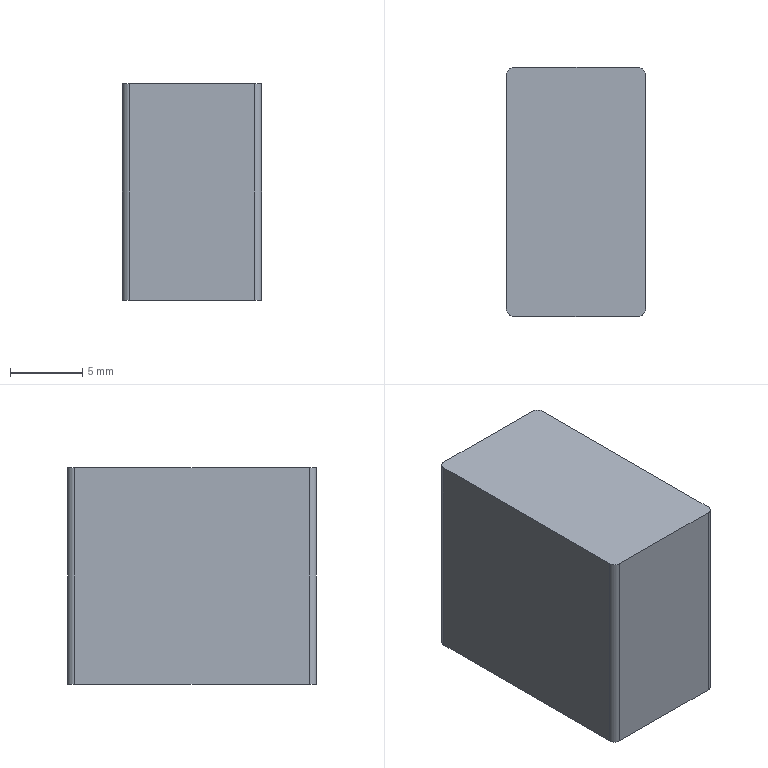Part | NX | features BREP 1 | 1 solid | 10 faces | box 9.615 x 17.2 x 15 mm | volume 2478 mm3 | plane 6 | cylinder 4 | commonest cylinder face diameters 1 x4
STEP:
#1=CARTESIAN_POINT('',(-4.308,8.6,-25.6));
#2=VERTEX_POINT('',#1);
#3=CARTESIAN_POINT('',(-4.808,8.1,-25.6));
#4=VERTEX_POINT('',#3);
#5=CARTESIAN_POINT('',(-4.308,8.1,-25.6));
#6=DIRECTION('',(0.,0.,1.));
#7=DIRECTION('',(1.,0.,0.));
#8=AXIS2_PLACEMENT_3D('',#5,#6,#7);
#9=CIRCLE('',#8,0.5);
#10=EDGE_CURVE('',#2,#4,#9,.T.);
#11=ORIENTED_EDGE('',*,*,#10,.F.);
#12=CARTESIAN_POINT('',(-4.308,8.6,-40.6));
#13=VERTEX_POINT('',#12);
#14=CARTESIAN_POINT('',(-4.308,8.6,-40.6));
#15=DIRECTION('',(0.,0.,1.));
#16=VECTOR('',#15,1000.);
#17=LINE('',#14,#16);
#18=EDGE_CURVE('',#13,#2,#17,.T.);
#19=ORIENTED_EDGE('',*,*,#18,.F.);
#20=CARTESIAN_POINT('',(-4.808,8.1,-40.6));
#21=VERTEX_POINT('',#20);
#22=CARTESIAN_POINT('',(-4.308,8.1,-40.6));
#23=DIRECTION('',(0.,0.,1.));
#24=DIRECTION('',(1.,0.,0.));
#25=AXIS2_PLACEMENT_3D('',#22,#23,#24);
#26=CIRCLE('',#25,0.5);
#27=EDGE_CURVE('',#13,#21,#26,.T.);
#28=ORIENTED_EDGE('',*,*,#27,.T.);
#29=CARTESIAN_POINT('',(-4.808,8.1,-40.6));
#30=DIRECTION('',(0.,0.,1.));
#31=VECTOR('',#30,1000.);
#32=LINE('',#29,#31);
#33=EDGE_CURVE('',#21,#4,#32,.T.);
#34=ORIENTED_EDGE('',*,*,#33,.T.);
#35=EDGE_LOOP('',(#11,#19,#28,#34));
#36=FACE_BOUND('',#35,.T.);
#37=CARTESIAN_POINT('',(-4.308,8.1,-40.6));
#38=DIRECTION('',(0.,0.,1.));
#39=DIRECTION('',(-1.,0.,0.));
#40=AXIS2_PLACEMENT_3D('',#37,#38,#39);
#41=CYLINDRICAL_SURFACE('',#40,0.5);
#42=ADVANCED_FACE('',(#36),#41,.T.);
#43=CARTESIAN_POINT('',(-4.808,-8.1,-25.6));
#44=VERTEX_POINT('',#43);
#45=CARTESIAN_POINT('',(-4.808,-8.1,-25.6));
#46=DIRECTION('',(0.,1.,0.));
#47=VECTOR('',#46,1000.);
#48=LINE('',#45,#47);
#49=EDGE_CURVE('',#44,#4,#48,.T.);
#50=ORIENTED_EDGE('',*,*,#49,.T.);
#51=ORIENTED_EDGE('',*,*,#33,.F.);
#52=CARTESIAN_POINT('',(-4.808,-8.1,-40.6));
#53=VERTEX_POINT('',#52);
#54=CARTESIAN_POINT('',(-4.808,-8.1,-40.6));
#55=DIRECTION('',(0.,1.,0.));
#56=VECTOR('',#55,1000.);
#57=LINE('',#54,#56);
#58=EDGE_CURVE('',#53,#21,#57,.T.);
#59=ORIENTED_EDGE('',*,*,#58,.F.);
#60=CARTESIAN_POINT('',(-4.808,-8.1,-40.6));
#61=DIRECTION('',(0.,0.,1.));
#62=VECTOR('',#61,1000.);
#63=LINE('',#60,#62);
#64=EDGE_CURVE('',#53,#44,#63,.T.);
#65=ORIENTED_EDGE('',*,*,#64,.T.);
#66=EDGE_LOOP('',(#50,#51,#59,#65));
#67=FACE_BOUND('',#66,.T.);
#68=CARTESIAN_POINT('',(-4.808,-8.1,-40.6));
#69=DIRECTION('',(1.,0.,0.));
#70=DIRECTION('',(0.,0.,1.));
#71=AXIS2_PLACEMENT_3D('',#68,#69,#70);
#72=PLANE('',#71);
#73=ADVANCED_FACE('',(#67),#72,.F.);
#74=CARTESIAN_POINT('',(-4.308,-8.6,-25.6));
#75=VERTEX_POINT('',#74);
#76=CARTESIAN_POINT('',(-4.308,-8.1,-25.6));
#77=DIRECTION('',(0.,0.,1.));
#78=DIRECTION('',(1.,0.,0.));
#79=AXIS2_PLACEMENT_3D('',#76,#77,#78);
#80=CIRCLE('',#79,0.5);
#81=EDGE_CURVE('',#44,#75,#80,.T.);
#82=ORIENTED_EDGE('',*,*,#81,.F.);
#83=ORIENTED_EDGE('',*,*,#64,.F.);
#84=CARTESIAN_POINT('',(-4.308,-8.6,-40.6));
#85=VERTEX_POINT('',#84);
#86=CARTESIAN_POINT('',(-4.308,-8.1,-40.6));
#87=DIRECTION('',(0.,0.,1.));
#88=DIRECTION('',(1.,0.,0.));
#89=AXIS2_PLACEMENT_3D('',#86,#87,#88);
#90=CIRCLE('',#89,0.5);
#91=EDGE_CURVE('',#53,#85,#90,.T.);
#92=ORIENTED_EDGE('',*,*,#91,.T.);
#93=CARTESIAN_POINT('',(-4.308,-8.6,-40.6));
#94=DIRECTION('',(0.,0.,1.));
#95=VECTOR('',#94,1000.);
#96=LINE('',#93,#95);
#97=EDGE_CURVE('',#85,#75,#96,.T.);
#98=ORIENTED_EDGE('',*,*,#97,.T.);
#99=EDGE_LOOP('',(#82,#83,#92,#98));
#100=FACE_BOUND('',#99,.T.);
#101=CARTESIAN_POINT('',(-4.308,-8.1,-40.6));
#102=DIRECTION('',(0.,0.,1.));
#103=DIRECTION('',(-1.,0.,0.));
#104=AXIS2_PLACEMENT_3D('',#101,#102,#103);
#105=CYLINDRICAL_SURFACE('',#104,0.5);
#106=ADVANCED_FACE('',(#100),#105,.T.);
#107=CARTESIAN_POINT('',(4.308,-8.6,-25.6));
#108=VERTEX_POINT('',#107);
#109=CARTESIAN_POINT('',(4.308,-8.6,-25.6));
#110=DIRECTION('',(-1.,0.,0.));
#111=VECTOR('',#110,1000.);
#112=LINE('',#109,#111);
#113=EDGE_CURVE('',#108,#75,#112,.T.);
#114=ORIENTED_EDGE('',*,*,#113,.T.);
#115=ORIENTED_EDGE('',*,*,#97,.F.);
#116=CARTESIAN_POINT('',(4.308,-8.6,-40.6));
#117=VERTEX_POINT('',#116);
#118=CARTESIAN_POINT('',(4.308,-8.6,-40.6));
#119=DIRECTION('',(-1.,0.,0.));
#120=VECTOR('',#119,1000.);
#121=LINE('',#118,#120);
#122=EDGE_CURVE('',#117,#85,#121,.T.);
#123=ORIENTED_EDGE('',*,*,#122,.F.);
#124=CARTESIAN_POINT('',(4.308,-8.6,-40.6));
#125=DIRECTION('',(0.,0.,1.));
#126=VECTOR('',#125,1000.);
#127=LINE('',#124,#126);
#128=EDGE_CURVE('',#117,#108,#127,.T.);
#129=ORIENTED_EDGE('',*,*,#128,.T.);
#130=EDGE_LOOP('',(#114,#115,#123,#129));
#131=FACE_BOUND('',#130,.T.);
#132=CARTESIAN_POINT('',(4.308,-8.6,-40.6));
#133=DIRECTION('',(0.,1.,0.));
#134=DIRECTION('',(0.,0.,-1.));
#135=AXIS2_PLACEMENT_3D('',#132,#133,#134);
#136=PLANE('',#135);
#137=ADVANCED_FACE('',(#131),#136,.F.);
#138=CARTESIAN_POINT('',(4.808,-8.1,-25.6));
#139=VERTEX_POINT('',#138);
#140=CARTESIAN_POINT('',(4.308,-8.1,-25.6));
#141=DIRECTION('',(0.,0.,1.));
#142=DIRECTION('',(1.,0.,0.));
#143=AXIS2_PLACEMENT_3D('',#140,#141,#142);
#144=CIRCLE('',#143,0.5);
#145=EDGE_CURVE('',#108,#139,#144,.T.);
#146=ORIENTED_EDGE('',*,*,#145,.F.);
#147=ORIENTED_EDGE('',*,*,#128,.F.);
#148=CARTESIAN_POINT('',(4.808,-8.1,-40.6));
#149=VERTEX_POINT('',#148);
#150=CARTESIAN_POINT('',(4.308,-8.1,-40.6));
#151=DIRECTION('',(0.,0.,1.));
#152=DIRECTION('',(1.,0.,0.));
#153=AXIS2_PLACEMENT_3D('',#150,#151,#152);
#154=CIRCLE('',#153,0.5);
#155=EDGE_CURVE('',#117,#149,#154,.T.);
#156=ORIENTED_EDGE('',*,*,#155,.T.);
#157=CARTESIAN_POINT('',(4.808,-8.1,-40.6));
#158=DIRECTION('',(0.,0.,1.));
#159=VECTOR('',#158,1000.);
#160=LINE('',#157,#159);
#161=EDGE_CURVE('',#149,#139,#160,.T.);
#162=ORIENTED_EDGE('',*,*,#161,.T.);
#163=EDGE_LOOP('',(#146,#147,#156,#162));
#164=FACE_BOUND('',#163,.T.);
#165=CARTESIAN_POINT('',(4.308,-8.1,-40.6));
#166=DIRECTION('',(0.,0.,1.));
#167=DIRECTION('',(-1.,0.,0.));
#168=AXIS2_PLACEMENT_3D('',#165,#166,#167);
#169=CYLINDRICAL_SURFACE('',#168,0.5);
#170=ADVANCED_FACE('',(#164),#169,.T.);
#171=CARTESIAN_POINT('',(4.808,8.1,-25.6));
#172=VERTEX_POINT('',#171);
#173=CARTESIAN_POINT('',(4.808,8.1,-25.6));
#174=DIRECTION('',(0.,-1.,0.));
#175=VECTOR('',#174,1000.);
#176=LINE('',#173,#175);
#177=EDGE_CURVE('',#172,#139,#176,.T.);
#178=ORIENTED_EDGE('',*,*,#177,.T.);
#179=ORIENTED_EDGE('',*,*,#161,.F.);
#180=CARTESIAN_POINT('',(4.808,8.1,-40.6));
#181=VERTEX_POINT('',#180);
#182=CARTESIAN_POINT('',(4.808,8.1,-40.6));
#183=DIRECTION('',(0.,-1.,0.));
#184=VECTOR('',#183,1000.);
#185=LINE('',#182,#184);
#186=EDGE_CURVE('',#181,#149,#185,.T.);
#187=ORIENTED_EDGE('',*,*,#186,.F.);
#188=CARTESIAN_POINT('',(4.808,8.1,-40.6));
#189=DIRECTION('',(0.,0.,1.));
#190=VECTOR('',#189,1000.);
#191=LINE('',#188,#190);
#192=EDGE_CURVE('',#181,#172,#191,.T.);
#193=ORIENTED_EDGE('',*,*,#192,.T.);
#194=EDGE_LOOP('',(#178,#179,#187,#193));
#195=FACE_BOUND('',#194,.T.);
#196=CARTESIAN_POINT('',(4.808,8.1,-40.6));
#197=DIRECTION('',(-1.,0.,0.));
#198=DIRECTION('',(0.,1.,0.));
#199=AXIS2_PLACEMENT_3D('',#196,#197,#198);
#200=PLANE('',#199);
#201=ADVANCED_FACE('',(#195),#200,.F.);
#202=CARTESIAN_POINT('',(4.308,8.6,-25.6));
#203=VERTEX_POINT('',#202);
#204=CARTESIAN_POINT('',(4.308,8.1,-25.6));
#205=DIRECTION('',(0.,0.,1.));
#206=DIRECTION('',(1.,0.,0.));
#207=AXIS2_PLACEMENT_3D('',#204,#205,#206);
#208=CIRCLE('',#207,0.5);
#209=EDGE_CURVE('',#172,#203,#208,.T.);
#210=ORIENTED_EDGE('',*,*,#209,.F.);
#211=ORIENTED_EDGE('',*,*,#192,.F.);
#212=CARTESIAN_POINT('',(4.308,8.6,-40.6));
#213=VERTEX_POINT('',#212);
#214=CARTESIAN_POINT('',(4.308,8.1,-40.6));
#215=DIRECTION('',(0.,0.,1.));
#216=DIRECTION('',(1.,0.,0.));
#217=AXIS2_PLACEMENT_3D('',#214,#215,#216);
#218=CIRCLE('',#217,0.5);
#219=EDGE_CURVE('',#181,#213,#218,.T.);
#220=ORIENTED_EDGE('',*,*,#219,.T.);
#221=CARTESIAN_POINT('',(4.308,8.6,-40.6));
#222=DIRECTION('',(0.,0.,1.));
#223=VECTOR('',#222,1000.);
#224=LINE('',#221,#223);
#225=EDGE_CURVE('',#213,#203,#224,.T.);
#226=ORIENTED_EDGE('',*,*,#225,.T.);
#227=EDGE_LOOP('',(#210,#211,#220,#226));
#228=FACE_BOUND('',#227,.T.);
#229=CARTESIAN_POINT('',(4.308,8.1,-40.6));
#230=DIRECTION('',(0.,0.,1.));
#231=DIRECTION('',(-1.,0.,0.));
#232=AXIS2_PLACEMENT_3D('',#229,#230,#231);
#233=CYLINDRICAL_SURFACE('',#232,0.5);
#234=ADVANCED_FACE('',(#228),#233,.T.);
#235=CARTESIAN_POINT('',(-4.308,8.6,-25.6));
#236=DIRECTION('',(1.,0.,0.));
#237=VECTOR('',#236,1000.);
#238=LINE('',#235,#237);
#239=EDGE_CURVE('',#2,#203,#238,.T.);
#240=ORIENTED_EDGE('',*,*,#239,.T.);
#241=ORIENTED_EDGE('',*,*,#225,.F.);
#242=CARTESIAN_POINT('',(-4.308,8.6,-40.6));
#243=DIRECTION('',(1.,0.,0.));
#244=VECTOR('',#243,1000.);
#245=LINE('',#242,#244);
#246=EDGE_CURVE('',#13,#213,#245,.T.);
#247=ORIENTED_EDGE('',*,*,#246,.F.);
#248=ORIENTED_EDGE('',*,*,#18,.T.);
#249=EDGE_LOOP('',(#240,#241,#247,#248));
#250=FACE_BOUND('',#249,.T.);
#251=CARTESIAN_POINT('',(-4.308,8.6,-40.6));
#252=DIRECTION('',(0.,-1.,0.));
#253=DIRECTION('',(0.,0.,1.));
#254=AXIS2_PLACEMENT_3D('',#251,#252,#253);
#255=PLANE('',#254);
#256=ADVANCED_FACE('',(#250),#255,.F.);
#257=ORIENTED_EDGE('',*,*,#27,.F.);
#258=ORIENTED_EDGE('',*,*,#246,.T.);
#259=ORIENTED_EDGE('',*,*,#219,.F.);
#260=ORIENTED_EDGE('',*,*,#186,.T.);
#261=ORIENTED_EDGE('',*,*,#155,.F.);
#262=ORIENTED_EDGE('',*,*,#122,.T.);
#263=ORIENTED_EDGE('',*,*,#91,.F.);
#264=ORIENTED_EDGE('',*,*,#58,.T.);
#265=EDGE_LOOP('',(#257,#258,#259,#260,#261,#262,#263,#264));
#266=FACE_BOUND('',#265,.T.);
#267=CARTESIAN_POINT('',(-4.308,8.1,-40.6));
#268=DIRECTION('',(0.,0.,1.));
#269=DIRECTION('',(-1.,0.,0.));
#270=AXIS2_PLACEMENT_3D('',#267,#268,#269);
#271=PLANE('',#270);
#272=ADVANCED_FACE('',(#266),#271,.F.);
#273=ORIENTED_EDGE('',*,*,#10,.T.);
#274=ORIENTED_EDGE('',*,*,#49,.F.);
#275=ORIENTED_EDGE('',*,*,#81,.T.);
#276=ORIENTED_EDGE('',*,*,#113,.F.);
#277=ORIENTED_EDGE('',*,*,#145,.T.);
#278=ORIENTED_EDGE('',*,*,#177,.F.);
#279=ORIENTED_EDGE('',*,*,#209,.T.);
#280=ORIENTED_EDGE('',*,*,#239,.F.);
#281=EDGE_LOOP('',(#273,#274,#275,#276,#277,#278,#279,#280));
#282=FACE_BOUND('',#281,.T.);
#283=CARTESIAN_POINT('',(-4.308,8.1,-25.6));
#284=DIRECTION('',(0.,0.,1.));
#285=DIRECTION('',(-1.,0.,0.));
#286=AXIS2_PLACEMENT_3D('',#283,#284,#285);
#287=PLANE('',#286);
#288=ADVANCED_FACE('',(#282),#287,.T.);
#289=CLOSED_SHELL('',(#42,#73,#106,#137,#170,#201,#234,#256,#272,#288));
#290=MANIFOLD_SOLID_BREP('',#289);
#291=(LENGTH_UNIT()NAMED_UNIT(*)SI_UNIT(.MILLI.,.METRE.));
#292=UNCERTAINTY_MEASURE_WITH_UNIT(LENGTH_MEASURE(0.00001),#291,'','');
#293=(NAMED_UNIT(*)PLANE_ANGLE_UNIT()SI_UNIT($,.RADIAN.));
#294=(NAMED_UNIT(*)SI_UNIT($,.STERADIAN.)SOLID_ANGLE_UNIT());
#295=(GEOMETRIC_REPRESENTATION_CONTEXT(3)GLOBAL_UNCERTAINTY_ASSIGNED_CONTEXT((#292))GLOBAL_UNIT_ASSIGNED_CONTEXT((#291,#293,#294))REPRESENTATION_CONTEXT('',''));
#296=ADVANCED_BREP_SHAPE_REPRESENTATION('',(#290),#295);